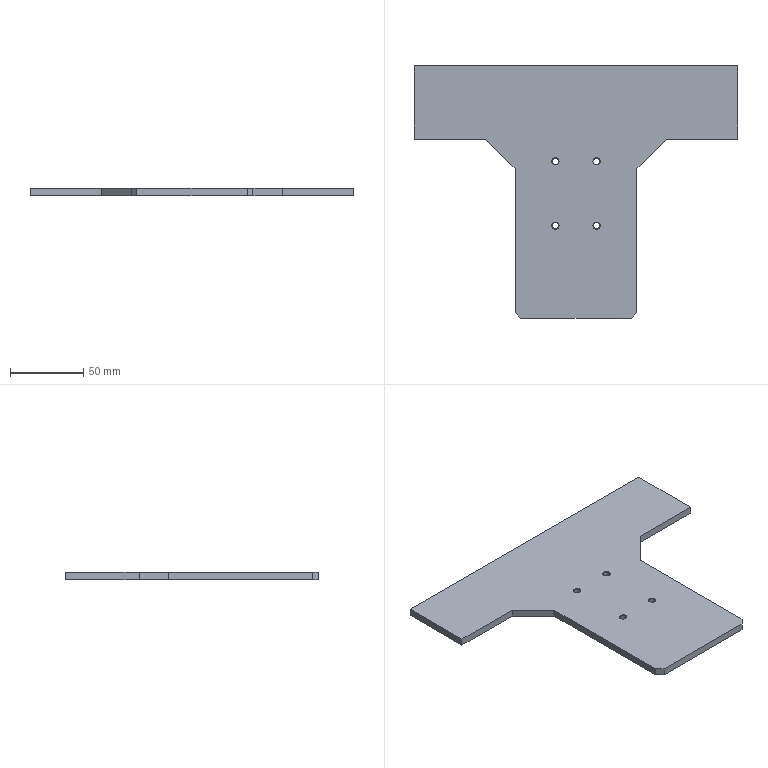Part | STEP file | Tube necking machine_id690_x_t | 1 solid | 26 faces | box 220 x 172 x 5 mm | volume 107264 mm3 | plane 14 | cone 8 | cylinder 4 | commonest cylinder face diameters 4.2 x4